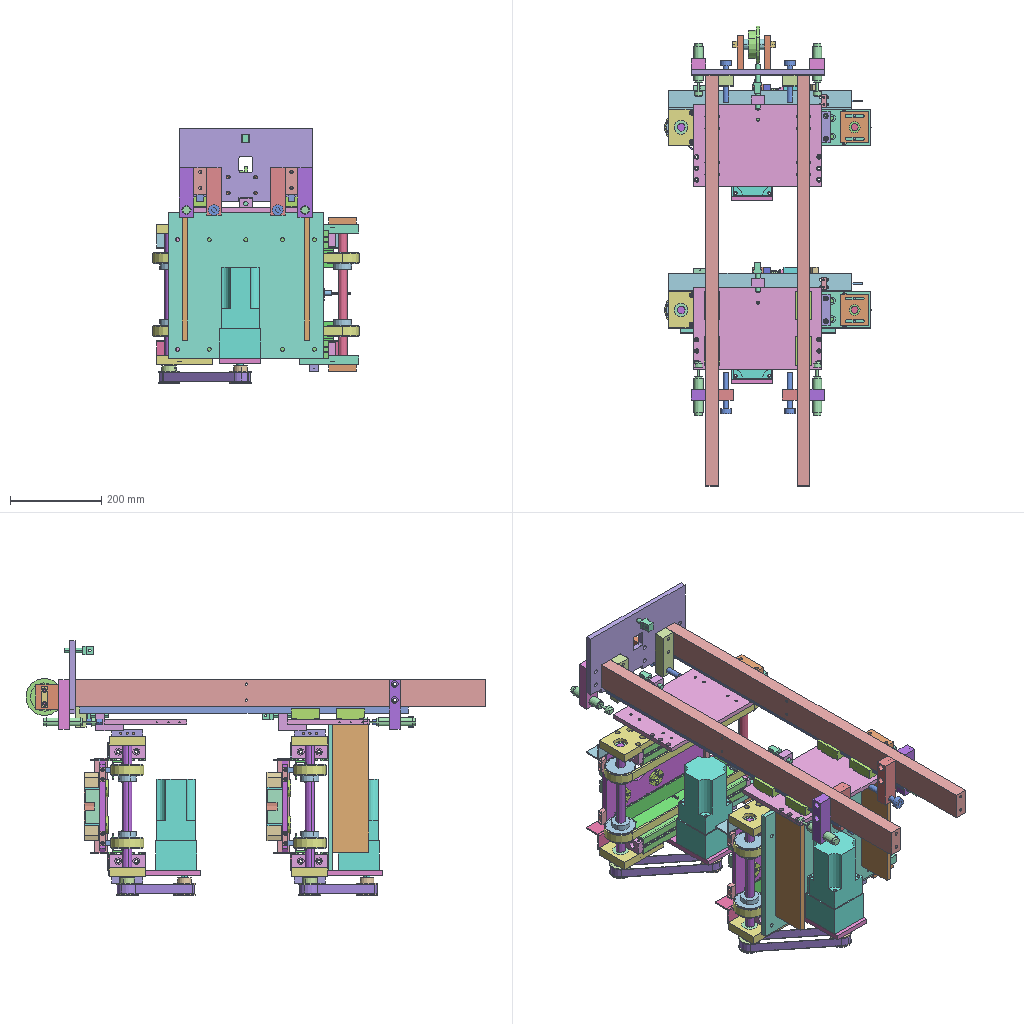Assembly | STEP file | 59 different items | 177 placed | box 451 x 1007 x 558 mm
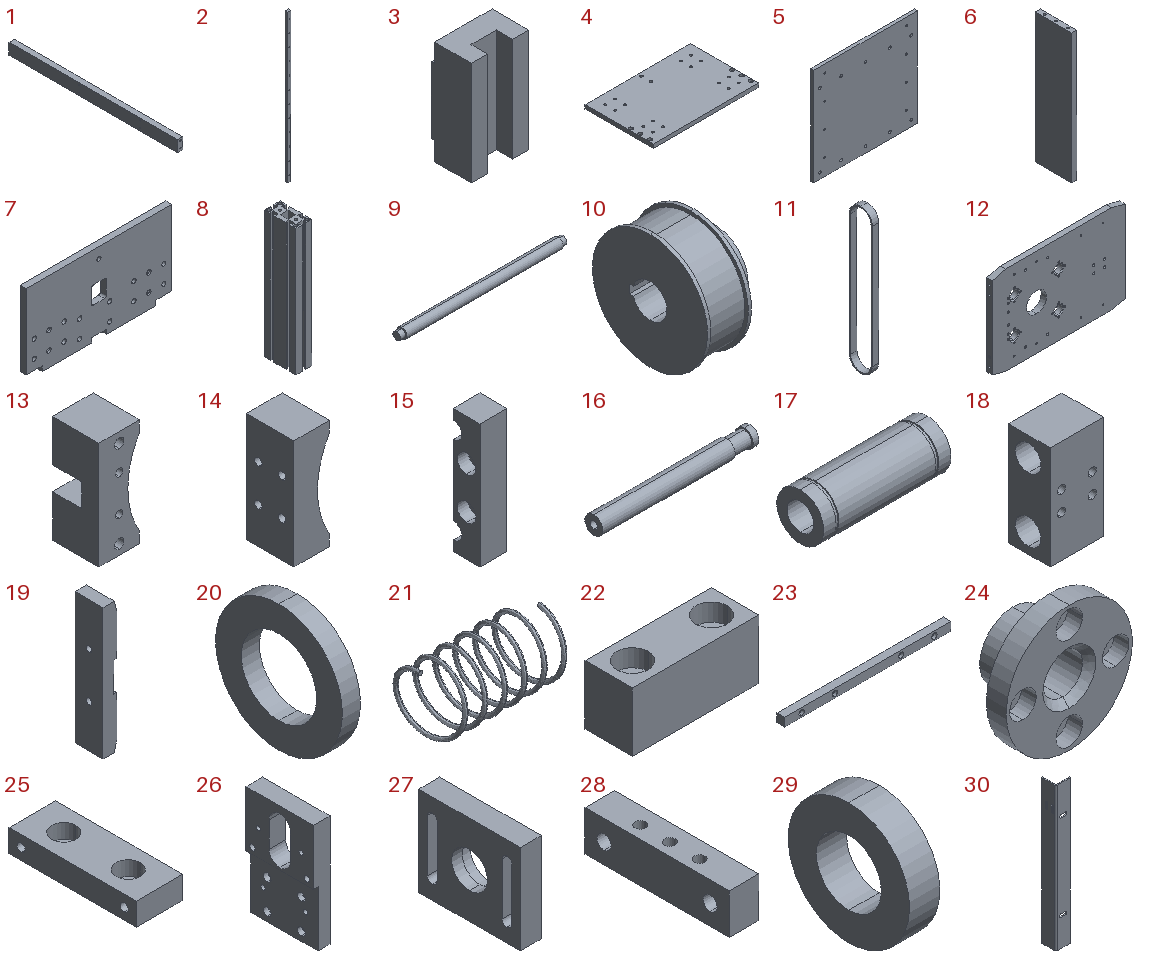Parts list (item | name | quantity | parent item | size | volume):
1 | PN_0056 (guide rail fixing plate) | x2 | - | 28 x 900 x 60 mm | 1504828 mm3
2 | PN_0023 (HGH15CA guide rail) | x2 | - | 15 x 14 x 720 mm | 146714 mm3
3 | PN_0004 (HGH15CA slider) | x4 | - | 34 x 23.7 x 61.4 mm | 38690 mm3
4 | PN_0009 (connecting block) | x2 | - | 280 x 180 x 10 mm | 491440 mm3
5 | PN_0013 (support block) | x1 | - | 340 x 10 x 320 mm | 1077927 mm3
6 | PN_0052 (inclined block) | x2 | - | 11 x 79 x 280 mm | 242077 mm3
7 | PN_0049 (fixing block) | x1 | - | 292 x 12 x 160 mm | 521488 mm3
8 | PN_0001 (cross beam) | x4 | - | 40 x 80 x 320 mm | 588947 mm3
9 | PN_0048 (auxiliary rotating shaft) | x2 | - | 328 x 20 x 20 mm | 99023 mm3
10 | PN_0002 (rotating wheel) | x8 | - | 38 x 68 x 68 mm | 87974 mm3
11 | PN_0031 (conveyor belt) | x4 | - | 20 x 72 x 452 mm | 77890 mm3
12 | PN_0003 (tooling plate) | x2 | in PN_0015 (tooling assembly, return) | 300 x 12 x 200 mm | 673943 mm3
13 | PN_0020 (half-round tube block) | x2 | in PN_0015 (tooling assembly, return) | 28 x 32 x 74 mm | 45440 mm3
14 | PN_0008 (movable half-round tube block) | x2 | in PN_0015 (spring press assembly) | 24 x 32 x 74 mm | 45434 mm3
15 | PN_0007 (clamp block) | x4 | in PN_0015 (spring press assembly) | 16 x 16 x 74 mm | 15676 mm3
16 | PN_0041 (guide rod) | x4 | in PN_0015 (spring press assembly) | 105 x 12 x 12 mm | 11156 mm3
17 | PN_0032 (linear bearing LM12LUU) | x4 | in PN_0015 (spring press assembly) | 57 x 21 x 21 mm | 13212 mm3
18 | PN_0010 (guide bushing seat) | x2 | in PN_0015 (spring press assembly) | 43.4 x 34 x 84 mm | 87676 mm3
19 | PN_0058 (connecting plate) | x2 | in PN_0015 (spring press assembly) | 16 x 32 x 150 mm | 73689 mm3
20 | PN_0018 (stop plate) | x4 | in PN_0015 (spring press assembly) | 3 x 21 x 21 mm | 670.926 mm3
21 | PN_0026 (spring) | x4 | in PN_0015 (spring press assembly) | 31 x 16 x 16 mm | 222.275 mm3
22 | PN_0044 (elastic rubber) | x4 | in PN_0015 (tooling assembly, return) | 32 x 12 x 15 mm | 4980 mm3
23 | PN_0030 (guide bar) | x4 | in PN_0015 (tooling assembly, return) | 250 x 12 x 12.5 mm | 36132 mm3
24 | PN_0024 (guide bushing) | x8 | in PN_0015 (tooling assembly, return) | 38 x 17 x 38 mm | 7268 mm3
25 | PN_0005 (reinforcing block) | x8 | - | 29 x 79 x 14 mm | 27118 mm3
26 | PN_0016 (connecting plate) | x4 | - | 19.5 x 79 x 130 mm | 136895 mm3
27 | PN_0055 (auxiliary rotating shaft seat) | x4 | - | 14 x 68 x 60 mm | 42344 mm3
28 | PN_0012 (fixing plate) | x4 | - | 14 x 68 x 19 mm | 15184 mm3
29 | PN_0039(ZZ6902) | x4 | - | 7 x 28 x 28 mm | 3073 mm3
30 | PN_0042 (stop side plate) | x2 | - | 40 x 40 x 400 mm | 89658 mm3
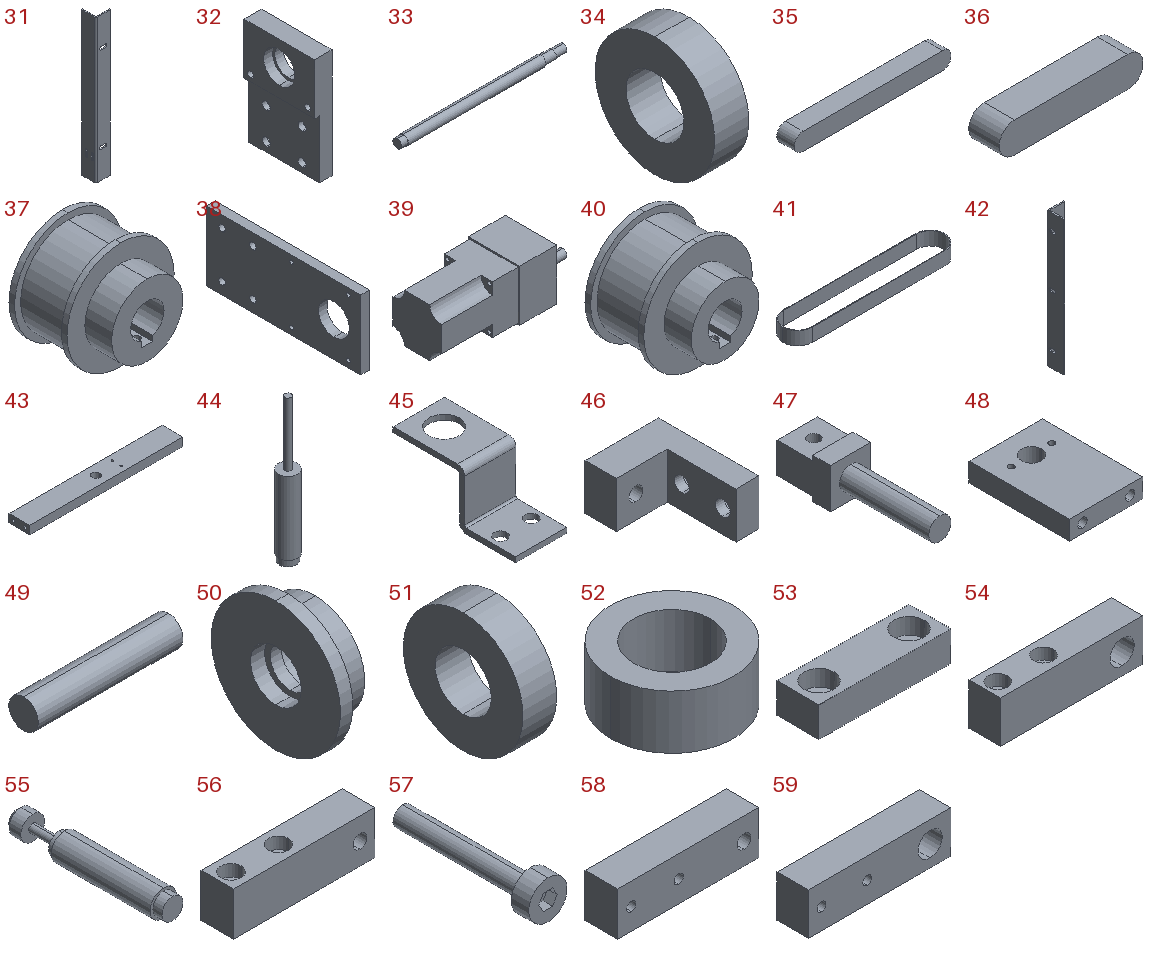31 | PN_0017 (stop side plate) | x2 | - | 40 x 40 x 400 mm | 89658 mm3
32 | PN_0027 (connecting plate) | x4 | - | 19.5 x 79 x 122 mm | 133748 mm3
33 | PN_0045 (main rotating shaft) | x2 | - | 325 x 20 x 20 mm | 94666 mm3
34 | PN_0054(ZZ6003) | x4 | - | 10 x 35 x 35 mm | 7351 mm3
35 | PN_0029 (key 5x5x40) | x8 | - | 45 x 5 x 5 mm | 1098 mm3
36 | PN_0028 (key 4x4x15) | x2 | - | 19 x 4 x 4 mm | 290.265 mm3
37 | PN_0038(ATP14L075)_ATP22XL050-A-H8 | x2 | - | 48 x 38 x 48 mm | 41242 mm3
38 | PN_0034 (motor mounting plate) | x2 | - | 11 x 200 x 90 mm | 180816 mm3
39 | PN_0043 (60W.1:15) | x2 | - | 238 x 90 x 90 mm | 1379919 mm3
40 | PN_0060(ATP14L075)_ATP22XL050-A-H8 | x2 | - | 48 x 38 x 48 mm | 40082 mm3
41 | PN_0006 (timing belt 210L, width 20, Z=56) | x2 | - | 244.45 x 44.45 x 20 mm | 10730 mm3
42 | PN_0021 (belt support block) | x4 | - | 40 x 40 x 340 mm | 77417 mm3
43 | PN_0057 (stop block) | x2 | - | 206 x 28 x 11 mm | 61677 mm3
44 | PN_0035 (M12-4 proximity switch) | x2 | - | 12 x 12 x 90 mm | 6055 mm3
45 | PN_0011 (proximity switch bracket) | x2 | - | 20 x 48 x 22 mm | 2356 mm3
46 | PN_0051 (connecting block) | x2 | - | 45 x 61 x 28 mm | 35599 mm3
47 | PN_0022 (hook) | x3 | - | 18 x 64 x 18 mm | 9415 mm3
48 | PN_0025 (support block) | x2 | - | 54 x 74 x 14 mm | 51598 mm3
49 | PN_0033 (shaft rod) | x1 | - | 74 x 15 x 15 mm | 13077 mm3
50 | PN_0053 (z=16,p=15.875 sprocket) | x1 | - | 25 x 81.37 x 81.37 mm | 74577 mm3
51 | PN_0059(ZZ6002) | x2 | - | 9 x 32 x 32 mm | 5648 mm3
52 | PN_0050 (stop plate) | x2 | - | 24 x 24 x 10.5 mm | 2895 mm3
53 | PN_0046 (stop block) | x2 | - | 44 x 14 x 10 mm | 5093 mm3
54 | PN_0040 (buffer fixing block) | x2 | - | 109 x 24 x 32 mm | 69208 mm3
55 | PN_0037 (hydraulic changer ACA2020) | x4 | - | 20 x 118 x 20 mm | 29167 mm3
56 | PN_0036 (positioning fixing block) | x2 | - | 104 x 24 x 32 mm | 69858 mm3
57 | PN_0019 (M12X60) | x4 | - | 24 x 91 x 24 mm | 13504 mm3
58 | PN_0047 (positioning fixing block) | x2 | - | 104 x 24 x 32 mm | 76168 mm3
59 | PN_0014 (buffer fixing block) | x2 | - | 109 x 24 x 32 mm | 75518 mm3
Placements (level | parent | child | x y z in mm | rotation matrix by rows):
1 | subassembly 2 | PN_0056 (guide rail fixing plate) | -56.042 -205.053 -30.0 | 1 0 0 0 1 0 0 0 1
1 | subassembly 2 | PN_0023 (HGH15CA guide rail) | -56.042 684.947 -30.0 | 1 0 0 0 0 1 0 -1 -0
1 | subassembly 2 | PN_0004 (HGH15CA slider) | -56.042 90.647 -34.3 | 1 0 0 0 0 1 0 -1 -0
1 | subassembly 2 | PN_0056 (guide rail fixing plate) | 143.958 -205.053 -30.0 | 1 0 0 0 1 0 0 0 1
1 | subassembly 2 | PN_0023 (HGH15CA guide rail) | 143.958 684.947 -30.0 | 1 0 0 0 0 1 0 -1 -0
1 | subassembly 2 | PN_0004 (HGH15CA slider) | 143.958 90.647 -34.3 | 1 0 0 0 0 1 0 -1 -0
1 | subassembly 2 | PN_0009 (connecting block) | 43.958 140.647 -68.0 | 1 0 0 0 1 0 0 0 1
1 | subassembly 2 | PN_0013 (support block) | 43.958 130.647 -68.0 | 1 0 0 0 1 0 0 0 1
1 | subassembly 2 | PN_0052 (inclined block) | 177.958 51.647 -68.0 | 1 0 0 0 1 0 0 0 1
1 | subassembly 2 | PN_0052 (inclined block) | -90.042 51.647 -68.0 | 1 0 0 0 1 0 0 0 1
1 | subassembly 2 | PN_0049 (fixing block) | 43.958 694.947 -45.0 | 1 0 0 0 1 0 0 0 1
1 | subassembly 2 | subassembly 3 | 105.958 169.332 -414.33 | 0 0 1 0 1 0 -1 0 0
2 | subassembly 3 | PN_0001 (cross beam) | -46.33 11.315 -200.0 | 1 0 0 0 1 0 0 0 1
2 | subassembly 3 | PN_0001 (cross beam) | -286.33 11.315 -200.0 | 1 0 0 0 1 0 0 0 1
2 | subassembly 3 | PN_0048 (auxiliary rotating shaft) | -330.33 11.315 150.0 | 1 0 0 0 0.9618 -0.2738 0 0.2738 0.9618
2 | subassembly 3 | PN_0002 (rotating wheel) | -73.33 11.315 150.0 | -1 0 0 0 0.9618 0.2738 0 0.2738 -0.9618
2 | subassembly 3 | PN_0031 (conveyor belt) | -86.33 11.315 150.0 | -1 0 0 0 -1 0 0 0 1
2 | subassembly 3 | PN_0002 (rotating wheel) | -259.33 11.315 150.0 | 1 0 0 0 0.9618 -0.2738 0 0.2738 0.9618
2 | subassembly 3 | PN_0031 (conveyor belt) | -246.33 11.315 150.0 | -1 0 0 0 -1 0 0 0 1
2 | subassembly 3 | PN_0015 (tooling assembly, return) | -166.33 74.53 -49.238 | 0 0 -1 0 1 0 1 0 0
3 | PN_0015 (tooling assembly, return) | PN_0003 (tooling plate) | -75.335 -9.216 -0.0 | 1 0 0 0 1 0 0 0 1
3 | PN_0015 (tooling assembly, return) | PN_0020 (half-round tube block) | -153.335 12.784 -0.0 | 1 0 0 0 1 0 0 0 1
3 | PN_0015 (tooling assembly, return) | PN_0015 (spring press assembly) | -58.515 11.875 -0.0 | -1 0 0 0 1 0 0 0 -1
4 | PN_0015 (spring press assembly) | PN_0008 (movable half-round tube block) | -57.18 2.909 -0.0 | 1 0 0 0 1 0 0 0 1
4 | PN_0015 (spring press assembly) | PN_0007 (clamp block) | -73.18 -13.091 0.0 | 1 0 0 0 1 0 0 0 1
4 | PN_0015 (spring press assembly) | PN_0007 (clamp block) | -73.18 18.909 -0.0 | 1 0 0 0 -1 0 0 0 -1
4 | PN_0015 (spring press assembly) | PN_0041 (guide rod) | -162.18 2.909 -26.0 | 1 0 0 0 0.9992 -0.03879 0 0.03879 0.9992
4 | PN_0015 (spring press assembly) | PN_0041 (guide rod) | -162.18 2.909 26.0 | 1 0 0 0 0.4218 -0.9067 0 0.9067 0.4218
4 | PN_0015 (spring press assembly) | PN_0032 (linear bearing LM12LUU) | -153.18 2.909 -26.0 | 1 0 0 0 1 0 0 0 1
4 | PN_0015 (spring press assembly) | PN_0032 (linear bearing LM12LUU) | -153.18 2.909 26.0 | 1 0 0 0 1 0 0 0 1
4 | PN_0015 (spring press assembly) | PN_0010 (guide bushing seat) | -124.68 -15.091 -0.0 | 1 0 0 0 1 0 0 0 1
4 | PN_0015 (spring press assembly) | PN_0058 (connecting plate) | -178.18 2.909 -0.0 | 1 0 0 0 1 0 0 0 1
4 | PN_0015 (spring press assembly) | PN_0018 (stop plate) | -96.18 2.909 26.0 | 1 0 0 0 1 0 0 0 1
4 | PN_0015 (spring press assembly) | PN_0018 (stop plate) | -96.18 2.909 -26.0 | 1 0 0 0 1 0 0 0 1
4 | PN_0015 (spring press assembly) | PN_0026 (spring) | -97.732 2.909 26.0 | 1 0 0 0 1 0 0 0 1
4 | PN_0015 (spring press assembly) | PN_0026 (spring) | -97.081 2.909 -26.0 | 1 0 0 0 0.9742 -0.2257 0 0.2257 0.9742
3 | PN_0015 (tooling assembly, return) | PN_0044 (elastic rubber) | -175.335 -9.216 -70.0 | 0 0 -1 0 1 0 1 0 0
3 | PN_0015 (tooling assembly, return) | PN_0044 (elastic rubber) | -175.335 -9.216 70.0 | 0 0 -1 0 1 0 1 0 0
3 | PN_0015 (tooling assembly, return) | PN_0030 (guide bar) | -25.335 -27.215 80.0 | 1 0 0 0 1 0 0 0 1
3 | PN_0015 (tooling assembly, return) | PN_0030 (guide bar) | -25.335 -27.215 -80.0 | 1 0 0 0 1 0 0 0 1
3 | PN_0015 (tooling assembly, return) | PN_0024 (guide bushing) | -125.335 -21.215 40.0 | 1 0 0 0 1 0 0 0 1
3 | PN_0015 (tooling assembly, return) | PN_0024 (guide bushing) | -125.335 -21.215 -40.0 | 1 0 0 0 1 0 0 0 1
3 | PN_0015 (tooling assembly, return) | PN_0024 (guide bushing) | -25.335 -21.215 40.0 | 1 0 0 0 1 0 0 0 1
3 | PN_0015 (tooling assembly, return) | PN_0024 (guide bushing) | -25.335 -21.215 -40.0 | 1 0 0 0 1 0 0 0 1
2 | subassembly 3 | PN_0005 (reinforcing block) | -46.33 11.315 120.0 | 1 0 0 0 1 0 0 0 1
2 | subassembly 3 | PN_0005 (reinforcing block) | -286.33 11.315 120.0 | 1 0 0 0 1 0 0 0 1
2 | subassembly 3 | PN_0005 (reinforcing block) | -46.33 11.315 -200.0 | -1 0 0 0 1 0 0 0 -1
2 | subassembly 3 | PN_0005 (reinforcing block) | -286.33 11.315 -200.0 | -1 0 0 0 1 0 0 0 -1
2 | subassembly 3 | subassembly 4 | -332.66 22.63 -80.0 | -1 0 0 0 -1 0 0 0 1
3 | subassembly 4 | PN_0016 (connecting plate) | -31.83 11.315 135.0 | 1 0 0 0 1 0 0 0 1
3 | subassembly 4 | PN_0055 (auxiliary rotating shaft seat) | -5.33 11.315 230.0 | -1 0 0 0 1 0 0 0 -1
3 | subassembly 4 | PN_0012 (fixing plate) | -5.33 11.315 167.0 | 1 0 0 0 1 0 0 0 1
3 | subassembly 4 | PN_0039(ZZ6902) | -12.33 11.315 230.0 | 1 0 0 0 1 0 0 0 1
2 | subassembly 3 | subassembly 4 | -0.0 0.0 -80.0 | 1 0 0 0 1 0 0 0 1
3 | subassembly 4 | PN_0016 (connecting plate) | -31.83 11.315 135.0 | 1 0 0 0 1 0 0 0 1
3 | subassembly 4 | PN_0055 (auxiliary rotating shaft seat) | -5.33 11.315 230.0 | -1 0 0 0 1 0 0 0 -1
3 | subassembly 4 | PN_0012 (fixing plate) | -5.33 11.315 167.0 | 1 0 0 0 1 0 0 0 1
3 | subassembly 4 | PN_0039(ZZ6902) | -12.33 11.315 230.0 | 1 0 0 0 1 0 0 0 1
2 | subassembly 3 | PN_0042 (stop side plate) | -66.33 51.315 143.0 | 1 0 0 0 1 0 0 0 1
2 | subassembly 3 | PN_0017 (stop side plate) | -266.33 51.315 -257.0 | -1 0 0 0 1 0 0 0 -1
2 | subassembly 3 | PN_0027 (connecting plate) | -31.83 11.315 -135.0 | 1 0 0 0 -1 0 0 0 -1
2 | subassembly 3 | PN_0027 (connecting plate) | -300.83 11.315 -135.0 | -1 0 0 0 1 0 0 0 -1
2 | subassembly 3 | PN_0045 (main rotating shaft) | -312.83 11.315 -230.0 | 1 0 0 0 0.9232 0.3844 0 -0.3844 0.9232
2 | subassembly 3 | PN_0054(ZZ6003) | -310.83 11.315 -230.0 | 1 0 0 0 1 0 0 0 1
2 | subassembly 3 | PN_0054(ZZ6003) | -31.83 11.315 -230.0 | 1 0 0 0 1 0 0 0 1
2 | subassembly 3 | PN_0029 (key 5x5x40) | -240.33 18.047 151.917 | 1 0 0 0 0.9618 -0.2738 0 0.2738 0.9618
2 | subassembly 3 | PN_0029 (key 5x5x40) | -92.33 18.047 151.917 | 1 0 0 0 0.9618 -0.2738 0 0.2738 0.9618
2 | subassembly 3 | PN_0029 (key 5x5x40) | -240.33 17.777 -232.69 | 1 0 0 0 0.9232 0.3844 0 -0.3844 0.9232
2 | subassembly 3 | PN_0029 (key 5x5x40) | -92.33 17.777 -232.69 | 1 0 0 0 0.9232 0.3844 0 -0.3844 0.9232
2 | subassembly 3 | PN_0002 (rotating wheel) | -73.33 11.315 -230.0 | -1 0 0 0 0.9232 -0.3844 0 -0.3844 -0.9232
2 | subassembly 3 | PN_0002 (rotating wheel) | -259.33 11.315 -230.0 | 1 0 0 0 0.9232 0.3844 0 -0.3844 0.9232
2 | subassembly 3 | PN_0028 (key 4x4x15) | 0.6702 15.931 -231.922 | 1 0 0 0 0.9232 0.3844 0 -0.3844 0.9232
2 | subassembly 3 | PN_0038(ATP14L075)_ATP22XL050-A-H8 | 4.67 11.315 -230.0 | 0 1 0 0.8409 0 0.5412 0.5412 0 -0.8409
2 | subassembly 3 | subassembly 5 | 16.937 -58.379 -73.875 | 1 0 0 0 1 0 0 0 1
3 | subassembly 5 | PN_0034 (motor mounting plate) | -37.767 -90.306 -0.0 | 1 0 0 0 1 0 0 0 1
3 | subassembly 5 | PN_0043 (60W.1:15) | -108.267 -37.306 -0.0 | 1 0 0 0 1 0 0 0 1
3 | subassembly 5 | PN_0060(ATP14L075)_ATP22XL050-A-H8 | -12.267 -55.306 0.0 | 0 1 0 -0.1427 0 -0.9898 -0.9898 0 0.1427
2 | subassembly 3 | PN_0006 (timing belt 210L, width 20, Z=56) | 15.217 -51.185 -151.938 | 0 0 1 0.625 0.7806 0 -0.7806 0.625 0
2 | subassembly 3 | PN_0021 (belt support block) | -266.33 3.315 130.0 | 1 0 0 0 1 0 0 0 1
2 | subassembly 3 | PN_0021 (belt support block) | -66.33 3.315 -210.0 | -1 0 0 0 1 0 0 0 -1
2 | subassembly 3 | PN_0057 (stop block) | -169.33 55.315 82.5 | 1 0 0 0 1 0 0 0 1
2 | subassembly 3 | PN_0035 (M12-4 proximity switch) | -169.33 69.315 76.451 | 0.7719 -0.6357 0 0.6357 0.7719 0 0 0 1
2 | subassembly 3 | PN_0011 (proximity switch bracket) | -131.33 69.315 90.0 | 0 -1 0 1 0 0 0 0 1
1 | subassembly 2 | PN_0004 (HGH15CA slider) | -56.042 190.647 -34.3 | 1 0 0 0 0 1 0 -1 -0
1 | subassembly 2 | PN_0004 (HGH15CA slider) | 143.958 190.647 -34.3 | 1 0 0 0 0 1 0 -1 -0
1 | subassembly 2 | PN_0051 (connecting block) | 43.958 188.647 -82.0 | 0 0 1 0 1 0 -1 0 0
1 | subassembly 2 | PN_0022 (hook) | 43.958 220.647 -49.0 | 0 0 1 0 1 0 -1 0 0
1 | subassembly 2 | subassembly 6 | 5.358 752.51 1.624 | 0 0 -1 0 1 0 1 0 0
2 | subassembly 6 | PN_0025 (support block) | -9.939 -45.563 -0.0 | 1 0 0 0 1 0 0 0 1
2 | subassembly 6 | PN_0025 (support block) | -9.939 -45.563 -60.0 | 1 0 0 0 1 0 0 0 1
2 | subassembly 6 | PN_0033 (shaft rod) | -9.939 9.437 -30.0 | 0 -0.03289 0.9995 0 0.9995 0.03289 -1 0 0
2 | subassembly 6 | subassembly 7 | -9.323 17.636 -38.04 | 0 0.07491 -0.9972 0 0.9972 0.07491 1 0 0
3 | subassembly 7 | PN_0053 (z=16,p=15.875 sprocket) | -4.46 -8.221 0.0 | 1 0 0 0 0.8869 -0.4619 0 0.4619 0.8869
3 | subassembly 7 | PN_0059(ZZ6002) | 11.54 -8.221 0.0 | 1 0 0 0 1 0 0 0 1
3 | subassembly 7 | PN_0059(ZZ6002) | -4.46 -8.221 -0.0 | 1 0 0 0 1 0 0 0 1
2 | subassembly 6 | PN_0050 (stop plate) | -9.939 9.437 -17.5 | 1 0 0 0 1 0 0 0 1
2 | subassembly 6 | PN_0050 (stop plate) | -9.939 9.437 -53.0 | 0.9993 0.03637 0 -0.03637 0.9993 0 0 0 1
2 | subassembly 6 | PN_0046 (stop block) | -9.939 9.437 7.0 | 1 0 0 0 1 0 0 0 1
2 | subassembly 6 | PN_0046 (stop block) | -9.939 9.437 -67.0 | -1 0 0 0 1 0 0 0 -1
1 | subassembly 2 | PN_0022 (hook) | 43.958 718.947 93.5 | 0 0 -1 0 -1 0 -1 0 0
1 | subassembly 2 | subassembly 8 | 173.958 -10.863 -72.058 | 0 0 1 0 1 0 -1 0 0
2 | subassembly 8 | PN_0040 (buffer fixing block) | -102.058 5.81 -0.0 | 1 0 0 0 1 0 0 0 1
2 | subassembly 8 | PN_0037 (hydraulic changer ACA2020) | -9.058 -40.34 -0.0 | 1 0 0 0 1 0 0 0 1
1 | subassembly 2 | subassembly 9 | 113.958 -3.218 -34.749 | 0 0 -1 0 -1 0 -1 0 -0
2 | subassembly 9 | PN_0036 (positioning fixing block) | -64.749 1.835 -0.0 | 1 0 0 0 1 0 0 0 1
2 | subassembly 9 | PN_0019 (M12X60) | 28.251 43.274 0.0 | -0.9457 0 0.3251 0 -1 0 0.3251 0 0.9457
1 | subassembly 2 | subassembly 8 | -86.042 -10.863 -72.058 | 0 0 1 0 1 0 -1 0 0
2 | subassembly 8 | PN_0040 (buffer fixing block) | -102.058 5.81 -0.0 | 1 0 0 0 1 0 0 0 1
2 | subassembly 8 | PN_0037 (hydraulic changer ACA2020) | -9.058 -40.34 -0.0 | 1 0 0 0 1 0 0 0 1
1 | subassembly 2 | subassembly 9 | -26.042 -3.218 -34.749 | 0 0 -1 0 -1 0 -1 0 0
2 | subassembly 9 | PN_0036 (positioning fixing block) | -64.749 1.835 -0.0 | 1 0 0 0 1 0 0 0 1
2 | subassembly 9 | PN_0019 (M12X60) | 28.251 43.274 0.0 | -0.9457 0 0.3251 0 -1 0 0.3251 0 0.9457
1 | subassembly 2 | subassembly 10 | 113.958 684.782 -34.749 | 0 0 -1 0 -1 0 -1 0 0
2 | subassembly 10 | PN_0047 (positioning fixing block) | -64.749 1.835 -0.0 | 1 0 0 0 1 0 0 0 1
2 | subassembly 10 | PN_0019 (M12X60) | 28.251 -42.058 0.0 | 0.9854 0 0.1701 0 1 0 -0.1701 0 0.9854
1 | subassembly 2 | subassembly 10 | -26.042 684.782 -34.749 | 0 0 -1 0 -1 0 -1 0 0
2 | subassembly 10 | PN_0047 (positioning fixing block) | -64.749 1.835 -0.0 | 1 0 0 0 1 0 0 0 1
2 | subassembly 10 | PN_0019 (M12X60) | 28.251 -42.058 0.0 | 0.9854 0 0.1701 0 1 0 -0.1701 0 0.9854
1 | subassembly 2 | subassembly 11 | 173.958 724.757 -72.058 | 0 0 -1 0 -1 0 -1 0 0
2 | subassembly 11 | PN_0014 (buffer fixing block) | -102.058 5.81 -0.0 | 1 0 0 0 1 0 0 0 1
2 | subassembly 11 | PN_0037 (hydraulic changer ACA2020) | -9.058 -40.34 -0.0 | 1 0 0 0 1 0 0 0 1
1 | subassembly 2 | subassembly 11 | -86.042 724.757 -72.058 | 0 0 -1 0 -1 0 -1 0 0
2 | subassembly 11 | PN_0014 (buffer fixing block) | -102.058 5.81 -0.0 | 1 0 0 0 1 0 0 0 1
2 | subassembly 11 | PN_0037 (hydraulic changer ACA2020) | -9.058 -40.34 -0.0 | 1 0 0 0 1 0 0 0 1
1 | subassembly 2 | PN_0051 (connecting block) | 43.958 588.647 -82.0 | 0 0 1 0 1 0 -1 0 0
1 | subassembly 2 | PN_0022 (hook) | 43.958 620.647 -49.0 | 0 0 1 0 1 0 -1 0 0
1 | subassembly 2 | PN_0009 (connecting block) | 43.958 540.647 -68.0 | 1 0 0 0 1 0 0 0 1
1 | subassembly 2 | subassembly 3 | 105.958 569.332 -414.33 | 0 0 1 0 1 0 -1 0 0
2 | subassembly 3 | PN_0001 (cross beam) | -46.33 11.315 -200.0 | 1 0 0 0 1 0 0 0 1
2 | subassembly 3 | PN_0001 (cross beam) | -286.33 11.315 -200.0 | 1 0 0 0 1 0 0 0 1
2 | subassembly 3 | PN_0048 (auxiliary rotating shaft) | -330.33 11.315 150.0 | 1 0 0 0 0.9618 -0.2738 0 0.2738 0.9618
2 | subassembly 3 | PN_0002 (rotating wheel) | -73.33 11.315 150.0 | -1 0 0 0 0.9618 0.2738 0 0.2738 -0.9618
2 | subassembly 3 | PN_0031 (conveyor belt) | -86.33 11.315 150.0 | -1 0 0 0 -1 0 0 0 1
2 | subassembly 3 | PN_0002 (rotating wheel) | -259.33 11.315 150.0 | 1 0 0 0 0.9618 -0.2738 0 0.2738 0.9618
2 | subassembly 3 | PN_0031 (conveyor belt) | -246.33 11.315 150.0 | -1 0 0 0 -1 0 0 0 1
2 | subassembly 3 | PN_0015 (tooling assembly, return) | -166.33 74.53 -49.238 | 0 0 -1 0 1 0 1 0 0
3 | PN_0015 (tooling assembly, return) | PN_0003 (tooling plate) | -75.335 -9.216 -0.0 | 1 0 0 0 1 0 0 0 1
3 | PN_0015 (tooling assembly, return) | PN_0020 (half-round tube block) | -153.335 12.784 -0.0 | 1 0 0 0 1 0 0 0 1
3 | PN_0015 (tooling assembly, return) | PN_0015 (spring press assembly) | -58.515 11.875 -0.0 | -1 0 0 0 1 0 0 0 -1
4 | PN_0015 (spring press assembly) | PN_0008 (movable half-round tube block) | -57.18 2.909 -0.0 | 1 0 0 0 1 0 0 0 1
4 | PN_0015 (spring press assembly) | PN_0007 (clamp block) | -73.18 -13.091 0.0 | 1 0 0 0 1 0 0 0 1
4 | PN_0015 (spring press assembly) | PN_0007 (clamp block) | -73.18 18.909 -0.0 | 1 0 0 0 -1 0 0 0 -1
4 | PN_0015 (spring press assembly) | PN_0041 (guide rod) | -162.18 2.909 -26.0 | 1 0 0 0 0.9992 -0.03879 0 0.03879 0.9992
4 | PN_0015 (spring press assembly) | PN_0041 (guide rod) | -162.18 2.909 26.0 | 1 0 0 0 0.4218 -0.9067 0 0.9067 0.4218
4 | PN_0015 (spring press assembly) | PN_0032 (linear bearing LM12LUU) | -153.18 2.909 -26.0 | 1 0 0 0 1 0 0 0 1
4 | PN_0015 (spring press assembly) | PN_0032 (linear bearing LM12LUU) | -153.18 2.909 26.0 | 1 0 0 0 1 0 0 0 1
4 | PN_0015 (spring press assembly) | PN_0010 (guide bushing seat) | -124.68 -15.091 -0.0 | 1 0 0 0 1 0 0 0 1
4 | PN_0015 (spring press assembly) | PN_0058 (connecting plate) | -178.18 2.909 -0.0 | 1 0 0 0 1 0 0 0 1
4 | PN_0015 (spring press assembly) | PN_0018 (stop plate) | -96.18 2.909 26.0 | 1 0 0 0 1 0 0 0 1
4 | PN_0015 (spring press assembly) | PN_0018 (stop plate) | -96.18 2.909 -26.0 | 1 0 0 0 1 0 0 0 1
4 | PN_0015 (spring press assembly) | PN_0026 (spring) | -97.732 2.909 26.0 | 1 0 0 0 1 0 0 0 1
4 | PN_0015 (spring press assembly) | PN_0026 (spring) | -97.081 2.909 -26.0 | 1 0 0 0 0.9742 -0.2257 0 0.2257 0.9742
3 | PN_0015 (tooling assembly, return) | PN_0044 (elastic rubber) | -175.335 -9.216 -70.0 | 0 0 -1 0 1 0 1 0 0
3 | PN_0015 (tooling assembly, return) | PN_0044 (elastic rubber) | -175.335 -9.216 70.0 | 0 0 -1 0 1 0 1 0 0
3 | PN_0015 (tooling assembly, return) | PN_0030 (guide bar) | -25.335 -27.215 80.0 | 1 0 0 0 1 0 0 0 1
3 | PN_0015 (tooling assembly, return) | PN_0030 (guide bar) | -25.335 -27.215 -80.0 | 1 0 0 0 1 0 0 0 1
3 | PN_0015 (tooling assembly, return) | PN_0024 (guide bushing) | -125.335 -21.215 40.0 | 1 0 0 0 1 0 0 0 1
3 | PN_0015 (tooling assembly, return) | PN_0024 (guide bushing) | -125.335 -21.215 -40.0 | 1 0 0 0 1 0 0 0 1
3 | PN_0015 (tooling assembly, return) | PN_0024 (guide bushing) | -25.335 -21.215 40.0 | 1 0 0 0 1 0 0 0 1
3 | PN_0015 (tooling assembly, return) | PN_0024 (guide bushing) | -25.335 -21.215 -40.0 | 1 0 0 0 1 0 0 0 1
2 | subassembly 3 | PN_0005 (reinforcing block) | -46.33 11.315 120.0 | 1 0 0 0 1 0 0 0 1
2 | subassembly 3 | PN_0005 (reinforcing block) | -286.33 11.315 120.0 | 1 0 0 0 1 0 0 0 1
2 | subassembly 3 | PN_0005 (reinforcing block) | -46.33 11.315 -200.0 | -1 0 0 0 1 0 0 0 -1
2 | subassembly 3 | PN_0005 (reinforcing block) | -286.33 11.315 -200.0 | -1 0 0 0 1 0 0 0 -1
2 | subassembly 3 | subassembly 4 | -332.66 22.63 -80.0 | -1 0 0 0 -1 0 0 0 1
3 | subassembly 4 | PN_0016 (connecting plate) | -31.83 11.315 135.0 | 1 0 0 0 1 0 0 0 1
3 | subassembly 4 | PN_0055 (auxiliary rotating shaft seat) | -5.33 11.315 230.0 | -1 0 0 0 1 0 0 0 -1
3 | subassembly 4 | PN_0012 (fixing plate) | -5.33 11.315 167.0 | 1 0 0 0 1 0 0 0 1
3 | subassembly 4 | PN_0039(ZZ6902) | -12.33 11.315 230.0 | 1 0 0 0 1 0 0 0 1
2 | subassembly 3 | subassembly 4 | -0.0 0.0 -80.0 | 1 0 0 0 1 0 0 0 1
3 | subassembly 4 | PN_0016 (connecting plate) | -31.83 11.315 135.0 | 1 0 0 0 1 0 0 0 1
3 | subassembly 4 | PN_0055 (auxiliary rotating shaft seat) | -5.33 11.315 230.0 | -1 0 0 0 1 0 0 0 -1
3 | subassembly 4 | PN_0012 (fixing plate) | -5.33 11.315 167.0 | 1 0 0 0 1 0 0 0 1
3 | subassembly 4 | PN_0039(ZZ6902) | -12.33 11.315 230.0 | 1 0 0 0 1 0 0 0 1
2 | subassembly 3 | PN_0042 (stop side plate) | -66.33 51.315 143.0 | 1 0 0 0 1 0 0 0 1
2 | subassembly 3 | PN_0017 (stop side plate) | -266.33 51.315 -257.0 | -1 0 0 0 1 0 0 0 -1
2 | subassembly 3 | PN_0027 (connecting plate) | -31.83 11.315 -135.0 | 1 0 0 0 -1 0 0 0 -1
2 | subassembly 3 | PN_0027 (connecting plate) | -300.83 11.315 -135.0 | -1 0 0 0 1 0 0 0 -1
2 | subassembly 3 | PN_0045 (main rotating shaft) | -312.83 11.315 -230.0 | 1 0 0 0 0.9232 0.3844 0 -0.3844 0.9232
2 | subassembly 3 | PN_0054(ZZ6003) | -310.83 11.315 -230.0 | 1 0 0 0 1 0 0 0 1
2 | subassembly 3 | PN_0054(ZZ6003) | -31.83 11.315 -230.0 | 1 0 0 0 1 0 0 0 1
2 | subassembly 3 | PN_0029 (key 5x5x40) | -240.33 18.047 151.917 | 1 0 0 0 0.9618 -0.2738 0 0.2738 0.9618
2 | subassembly 3 | PN_0029 (key 5x5x40) | -92.33 18.047 151.917 | 1 0 0 0 0.9618 -0.2738 0 0.2738 0.9618
2 | subassembly 3 | PN_0029 (key 5x5x40) | -240.33 17.777 -232.69 | 1 0 0 0 0.9232 0.3844 0 -0.3844 0.9232
2 | subassembly 3 | PN_0029 (key 5x5x40) | -92.33 17.777 -232.69 | 1 0 0 0 0.9232 0.3844 0 -0.3844 0.9232
2 | subassembly 3 | PN_0002 (rotating wheel) | -73.33 11.315 -230.0 | -1 0 0 0 0.9232 -0.3844 0 -0.3844 -0.9232
2 | subassembly 3 | PN_0002 (rotating wheel) | -259.33 11.315 -230.0 | 1 0 0 0 0.9232 0.3844 0 -0.3844 0.9232
2 | subassembly 3 | PN_0028 (key 4x4x15) | 0.6702 15.931 -231.922 | 1 0 0 0 0.9232 0.3844 0 -0.3844 0.9232
2 | subassembly 3 | PN_0038(ATP14L075)_ATP22XL050-A-H8 | 4.67 11.315 -230.0 | 0 1 0 0.8409 0 0.5412 0.5412 0 -0.8409
2 | subassembly 3 | subassembly 5 | 16.937 -58.379 -73.875 | 1 0 0 0 1 0 0 0 1
3 | subassembly 5 | PN_0034 (motor mounting plate) | -37.767 -90.306 -0.0 | 1 0 0 0 1 0 0 0 1
3 | subassembly 5 | PN_0043 (60W.1:15) | -108.267 -37.306 -0.0 | 1 0 0 0 1 0 0 0 1
3 | subassembly 5 | PN_0060(ATP14L075)_ATP22XL050-A-H8 | -12.267 -55.306 0.0 | 0 1 0 -0.1427 0 -0.9898 -0.9898 0 0.1427
2 | subassembly 3 | PN_0006 (timing belt 210L, width 20, Z=56) | 15.217 -51.185 -151.938 | 0 0 1 0.625 0.7806 0 -0.7806 0.625 0
2 | subassembly 3 | PN_0021 (belt support block) | -266.33 3.315 130.0 | 1 0 0 0 1 0 0 0 1
2 | subassembly 3 | PN_0021 (belt support block) | -66.33 3.315 -210.0 | -1 0 0 0 1 0 0 0 -1
2 | subassembly 3 | PN_0057 (stop block) | -169.33 55.315 82.5 | 1 0 0 0 1 0 0 0 1
2 | subassembly 3 | PN_0035 (M12-4 proximity switch) | -169.33 69.315 76.451 | 0.7719 -0.6357 0 0.6357 0.7719 0 0 0 1
2 | subassembly 3 | PN_0011 (proximity switch bracket) | -131.33 69.315 90.0 | 0 -1 0 1 0 0 0 0 1